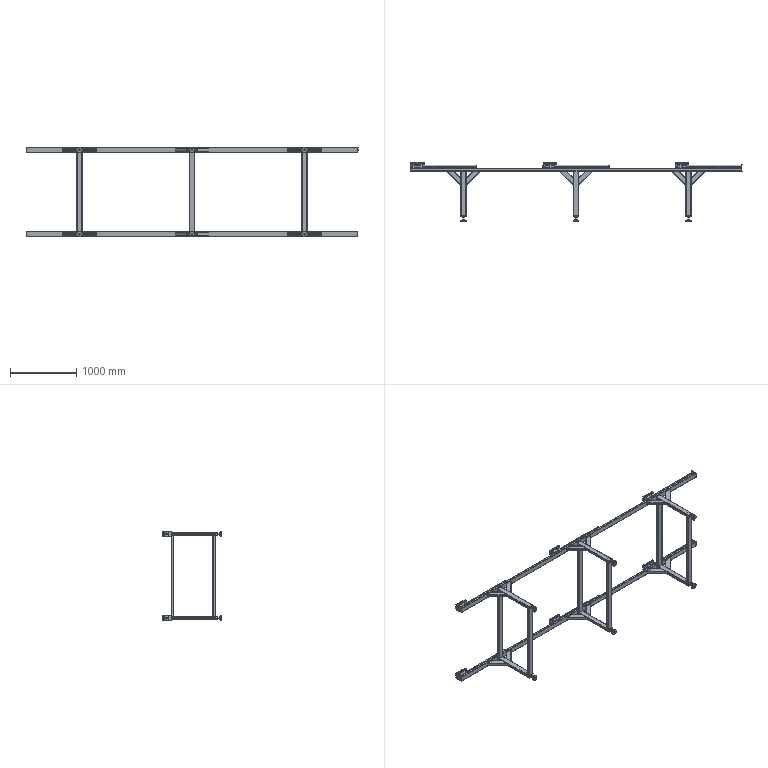Part | SolidWorks | features ReferencePattern 16, LocalLPattern 1 | 66 solids | 3238 faces | volume 30307292 mm3 | cylinder 1514 | plane 1052 | torus 246 | cone 168 | sphere 156 | spline 102 | commonest cylinder face diameters 0.7 x264 0.35 x204 6.6 x120 6 x104 12 x104 9 x96